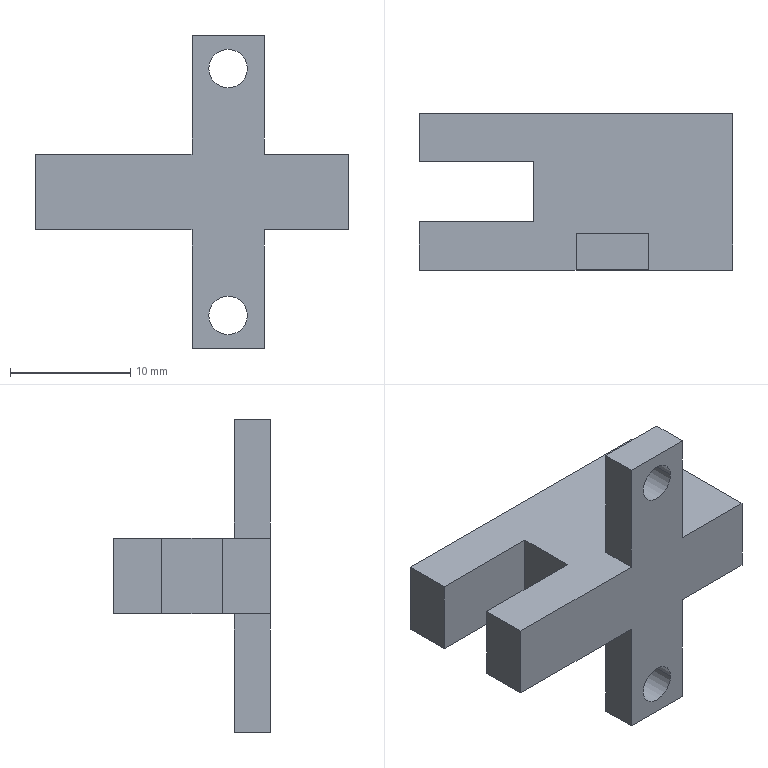Part | STEP file | PN_0010 photoelectric switch EE-SX672, Omron | 1 solid | 22 faces | box 26 x 13 x 26 mm | volume 2136 mm3 | plane 18 | cylinder 4 | commonest cylinder face diameters 3.2 x4